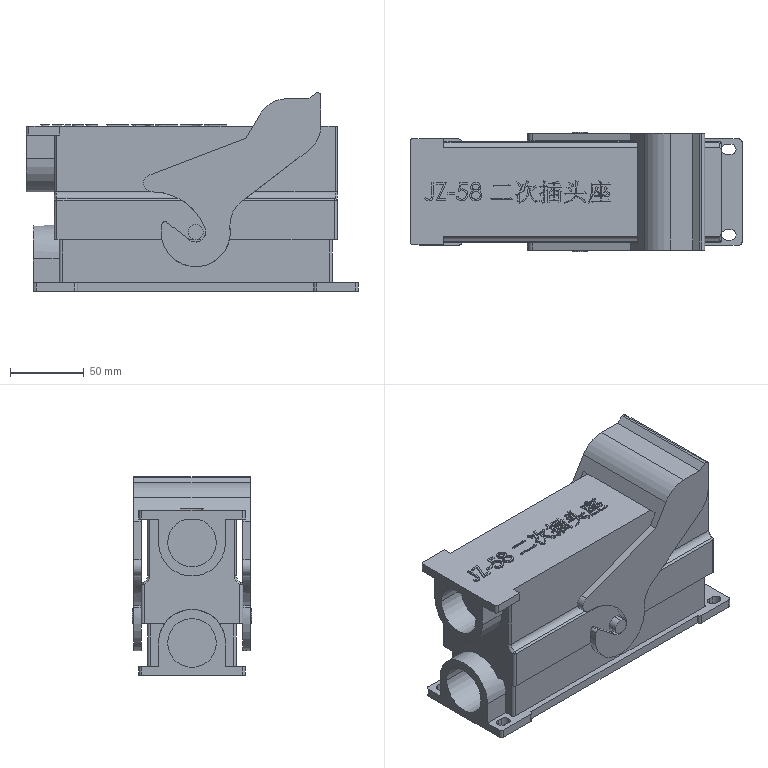Part | STEP file | JZ-58 secondary plug socket | 1 solid | 426 faces | box 225 x 81 x 134.749 mm | volume 1282541 mm3 | plane 266 | spline 85 | cylinder 71 | cone 4 | commonest cylinder face diameters 4 x23 7 x12 33 x7 40 x5 10.354 x4 11.636 x3